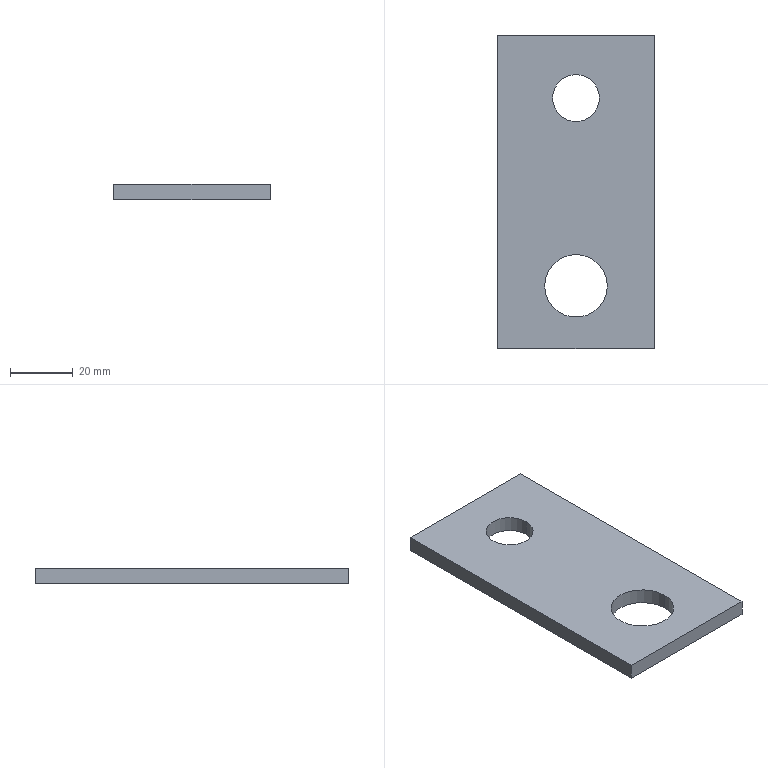Part | SolidWorks | features Extrusion 1, ICE 1 | 1 solid | 10 faces | box 50 x 100 x 5 mm | volume 22546 mm3 | plane 6 | cylinder 4 | commonest cylinder face diameters 15 x2 20 x2
STEP:
#1=CARTESIAN_POINT('',(-7.5,30.,0.));
#2=VERTEX_POINT('',#1);
#3=CARTESIAN_POINT('',(7.5,30.,0.));
#4=VERTEX_POINT('',#3);
#5=CARTESIAN_POINT('',(0.,30.,0.));
#6=DIRECTION('',(0.,0.,1.));
#7=DIRECTION('',(1.,0.,0.));
#8=AXIS2_PLACEMENT_3D('',#5,#6,#7);
#9=CIRCLE('',#8,7.5);
#10=EDGE_CURVE('',#2,#4,#9,.T.);
#11=ORIENTED_EDGE('',*,*,#10,.F.);
#12=CARTESIAN_POINT('',(-7.5,30.,5.));
#13=VERTEX_POINT('',#12);
#14=CARTESIAN_POINT('',(-7.5,30.,0.));
#15=DIRECTION('',(0.,0.,1.));
#16=VECTOR('',#15,1000.);
#17=LINE('',#14,#16);
#18=EDGE_CURVE('',#2,#13,#17,.T.);
#19=ORIENTED_EDGE('',*,*,#18,.T.);
#20=CARTESIAN_POINT('',(7.5,30.,5.));
#21=VERTEX_POINT('',#20);
#22=CARTESIAN_POINT('',(0.,30.,5.));
#23=DIRECTION('',(0.,0.,1.));
#24=DIRECTION('',(1.,0.,0.));
#25=AXIS2_PLACEMENT_3D('',#22,#23,#24);
#26=CIRCLE('',#25,7.5);
#27=EDGE_CURVE('',#13,#21,#26,.T.);
#28=ORIENTED_EDGE('',*,*,#27,.T.);
#29=CARTESIAN_POINT('',(7.5,30.,0.));
#30=DIRECTION('',(0.,0.,1.));
#31=VECTOR('',#30,1000.);
#32=LINE('',#29,#31);
#33=EDGE_CURVE('',#4,#21,#32,.T.);
#34=ORIENTED_EDGE('',*,*,#33,.F.);
#35=EDGE_LOOP('',(#11,#19,#28,#34));
#36=FACE_OUTER_BOUND('',#35,.T.);
#37=CARTESIAN_POINT('',(0.,30.,0.));
#38=DIRECTION('',(0.,0.,1.));
#39=DIRECTION('',(1.,0.,0.));
#40=AXIS2_PLACEMENT_3D('',#37,#38,#39);
#41=CYLINDRICAL_SURFACE('',#40,7.5);
#42=ADVANCED_FACE('',(#36),#41,.F.);
#43=CARTESIAN_POINT('',(-10.,-30.,0.));
#44=VERTEX_POINT('',#43);
#45=CARTESIAN_POINT('',(10.,-30.,0.));
#46=VERTEX_POINT('',#45);
#47=CARTESIAN_POINT('',(0.,-30.,0.));
#48=DIRECTION('',(0.,0.,1.));
#49=DIRECTION('',(1.,0.,0.));
#50=AXIS2_PLACEMENT_3D('',#47,#48,#49);
#51=CIRCLE('',#50,10.);
#52=EDGE_CURVE('',#44,#46,#51,.T.);
#53=ORIENTED_EDGE('',*,*,#52,.F.);
#54=CARTESIAN_POINT('',(-10.,-30.,5.));
#55=VERTEX_POINT('',#54);
#56=CARTESIAN_POINT('',(-10.,-30.,0.));
#57=DIRECTION('',(0.,0.,1.));
#58=VECTOR('',#57,1000.);
#59=LINE('',#56,#58);
#60=EDGE_CURVE('',#44,#55,#59,.T.);
#61=ORIENTED_EDGE('',*,*,#60,.T.);
#62=CARTESIAN_POINT('',(10.,-30.,5.));
#63=VERTEX_POINT('',#62);
#64=CARTESIAN_POINT('',(0.,-30.,5.));
#65=DIRECTION('',(0.,0.,1.));
#66=DIRECTION('',(1.,0.,0.));
#67=AXIS2_PLACEMENT_3D('',#64,#65,#66);
#68=CIRCLE('',#67,10.);
#69=EDGE_CURVE('',#55,#63,#68,.T.);
#70=ORIENTED_EDGE('',*,*,#69,.T.);
#71=CARTESIAN_POINT('',(10.,-30.,0.));
#72=DIRECTION('',(0.,0.,1.));
#73=VECTOR('',#72,1000.);
#74=LINE('',#71,#73);
#75=EDGE_CURVE('',#46,#63,#74,.T.);
#76=ORIENTED_EDGE('',*,*,#75,.F.);
#77=EDGE_LOOP('',(#53,#61,#70,#76));
#78=FACE_OUTER_BOUND('',#77,.T.);
#79=CARTESIAN_POINT('',(0.,-30.,0.));
#80=DIRECTION('',(0.,0.,1.));
#81=DIRECTION('',(1.,0.,0.));
#82=AXIS2_PLACEMENT_3D('',#79,#80,#81);
#83=CYLINDRICAL_SURFACE('',#82,10.);
#84=ADVANCED_FACE('',(#78),#83,.F.);
#85=CARTESIAN_POINT('',(-25.,50.,0.));
#86=VERTEX_POINT('',#85);
#87=CARTESIAN_POINT('',(-25.,-50.,0.));
#88=VERTEX_POINT('',#87);
#89=CARTESIAN_POINT('',(-25.,50.,0.));
#90=DIRECTION('',(0.,-1.,0.));
#91=VECTOR('',#90,1000.);
#92=LINE('',#89,#91);
#93=EDGE_CURVE('',#86,#88,#92,.T.);
#94=ORIENTED_EDGE('',*,*,#93,.T.);
#95=CARTESIAN_POINT('',(-25.,-50.,5.));
#96=VERTEX_POINT('',#95);
#97=CARTESIAN_POINT('',(-25.,-50.,5.));
#98=DIRECTION('',(0.,0.,-1.));
#99=VECTOR('',#98,1000.);
#100=LINE('',#97,#99);
#101=EDGE_CURVE('',#96,#88,#100,.T.);
#102=ORIENTED_EDGE('',*,*,#101,.F.);
#103=CARTESIAN_POINT('',(-25.,50.,5.));
#104=VERTEX_POINT('',#103);
#105=CARTESIAN_POINT('',(-25.,50.,5.));
#106=DIRECTION('',(0.,-1.,0.));
#107=VECTOR('',#106,1000.);
#108=LINE('',#105,#107);
#109=EDGE_CURVE('',#104,#96,#108,.T.);
#110=ORIENTED_EDGE('',*,*,#109,.F.);
#111=CARTESIAN_POINT('',(-25.,50.,5.));
#112=DIRECTION('',(0.,0.,-1.));
#113=VECTOR('',#112,1000.);
#114=LINE('',#111,#113);
#115=EDGE_CURVE('',#104,#86,#114,.T.);
#116=ORIENTED_EDGE('',*,*,#115,.T.);
#117=EDGE_LOOP('',(#94,#102,#110,#116));
#118=FACE_OUTER_BOUND('',#117,.T.);
#119=CARTESIAN_POINT('',(-25.,50.,5.));
#120=DIRECTION('',(1.,0.,0.));
#121=DIRECTION('',(0.,1.,0.));
#122=AXIS2_PLACEMENT_3D('',#119,#120,#121);
#123=PLANE('',#122);
#124=ADVANCED_FACE('',(#118),#123,.F.);
#125=CARTESIAN_POINT('',(25.,-50.,0.));
#126=VERTEX_POINT('',#125);
#127=CARTESIAN_POINT('',(25.,-50.,0.));
#128=DIRECTION('',(1.,0.,0.));
#129=VECTOR('',#128,1000.);
#130=LINE('',#127,#129);
#131=EDGE_CURVE('',#88,#126,#130,.T.);
#132=ORIENTED_EDGE('',*,*,#131,.T.);
#133=CARTESIAN_POINT('',(25.,-50.,5.));
#134=VERTEX_POINT('',#133);
#135=CARTESIAN_POINT('',(25.,-50.,5.));
#136=DIRECTION('',(0.,0.,-1.));
#137=VECTOR('',#136,1000.);
#138=LINE('',#135,#137);
#139=EDGE_CURVE('',#134,#126,#138,.T.);
#140=ORIENTED_EDGE('',*,*,#139,.F.);
#141=CARTESIAN_POINT('',(25.,-50.,5.));
#142=DIRECTION('',(1.,0.,0.));
#143=VECTOR('',#142,1000.);
#144=LINE('',#141,#143);
#145=EDGE_CURVE('',#96,#134,#144,.T.);
#146=ORIENTED_EDGE('',*,*,#145,.F.);
#147=ORIENTED_EDGE('',*,*,#101,.T.);
#148=EDGE_LOOP('',(#132,#140,#146,#147));
#149=FACE_OUTER_BOUND('',#148,.T.);
#150=CARTESIAN_POINT('',(25.,-50.,5.));
#151=DIRECTION('',(0.,1.,0.));
#152=DIRECTION('',(0.,0.,1.));
#153=AXIS2_PLACEMENT_3D('',#150,#151,#152);
#154=PLANE('',#153);
#155=ADVANCED_FACE('',(#149),#154,.F.);
#156=CARTESIAN_POINT('',(25.,50.,0.));
#157=VERTEX_POINT('',#156);
#158=CARTESIAN_POINT('',(25.,50.,0.));
#159=DIRECTION('',(0.,1.,0.));
#160=VECTOR('',#159,1000.);
#161=LINE('',#158,#160);
#162=EDGE_CURVE('',#126,#157,#161,.T.);
#163=ORIENTED_EDGE('',*,*,#162,.T.);
#164=CARTESIAN_POINT('',(25.,50.,5.));
#165=VERTEX_POINT('',#164);
#166=CARTESIAN_POINT('',(25.,50.,5.));
#167=DIRECTION('',(0.,0.,-1.));
#168=VECTOR('',#167,1000.);
#169=LINE('',#166,#168);
#170=EDGE_CURVE('',#165,#157,#169,.T.);
#171=ORIENTED_EDGE('',*,*,#170,.F.);
#172=CARTESIAN_POINT('',(25.,50.,5.));
#173=DIRECTION('',(0.,1.,0.));
#174=VECTOR('',#173,1000.);
#175=LINE('',#172,#174);
#176=EDGE_CURVE('',#134,#165,#175,.T.);
#177=ORIENTED_EDGE('',*,*,#176,.F.);
#178=ORIENTED_EDGE('',*,*,#139,.T.);
#179=EDGE_LOOP('',(#163,#171,#177,#178));
#180=FACE_OUTER_BOUND('',#179,.T.);
#181=CARTESIAN_POINT('',(25.,50.,5.));
#182=DIRECTION('',(-1.,0.,0.));
#183=DIRECTION('',(0.,-1.,0.));
#184=AXIS2_PLACEMENT_3D('',#181,#182,#183);
#185=PLANE('',#184);
#186=ADVANCED_FACE('',(#180),#185,.F.);
#187=CARTESIAN_POINT('',(25.,50.,0.));
#188=DIRECTION('',(-1.,0.,0.));
#189=VECTOR('',#188,1000.);
#190=LINE('',#187,#189);
#191=EDGE_CURVE('',#157,#86,#190,.T.);
#192=ORIENTED_EDGE('',*,*,#191,.T.);
#193=ORIENTED_EDGE('',*,*,#115,.F.);
#194=CARTESIAN_POINT('',(25.,50.,5.));
#195=DIRECTION('',(-1.,0.,0.));
#196=VECTOR('',#195,1000.);
#197=LINE('',#194,#196);
#198=EDGE_CURVE('',#165,#104,#197,.T.);
#199=ORIENTED_EDGE('',*,*,#198,.F.);
#200=ORIENTED_EDGE('',*,*,#170,.T.);
#201=EDGE_LOOP('',(#192,#193,#199,#200));
#202=FACE_OUTER_BOUND('',#201,.T.);
#203=CARTESIAN_POINT('',(25.,50.,5.));
#204=DIRECTION('',(0.,-1.,0.));
#205=DIRECTION('',(0.,0.,-1.));
#206=AXIS2_PLACEMENT_3D('',#203,#204,#205);
#207=PLANE('',#206);
#208=ADVANCED_FACE('',(#202),#207,.F.);
#209=CARTESIAN_POINT('',(0.,30.,5.));
#210=DIRECTION('',(0.,0.,1.));
#211=DIRECTION('',(1.,0.,0.));
#212=AXIS2_PLACEMENT_3D('',#209,#210,#211);
#213=CIRCLE('',#212,7.5);
#214=EDGE_CURVE('',#21,#13,#213,.T.);
#215=ORIENTED_EDGE('',*,*,#214,.F.);
#216=ORIENTED_EDGE('',*,*,#27,.F.);
#217=EDGE_LOOP('',(#215,#216));
#218=FACE_BOUND('',#217,.T.);
#219=CARTESIAN_POINT('',(0.,-30.,5.));
#220=DIRECTION('',(0.,0.,1.));
#221=DIRECTION('',(1.,0.,0.));
#222=AXIS2_PLACEMENT_3D('',#219,#220,#221);
#223=CIRCLE('',#222,10.);
#224=EDGE_CURVE('',#63,#55,#223,.T.);
#225=ORIENTED_EDGE('',*,*,#224,.F.);
#226=ORIENTED_EDGE('',*,*,#69,.F.);
#227=EDGE_LOOP('',(#225,#226));
#228=FACE_BOUND('',#227,.T.);
#229=ORIENTED_EDGE('',*,*,#109,.T.);
#230=ORIENTED_EDGE('',*,*,#145,.T.);
#231=ORIENTED_EDGE('',*,*,#176,.T.);
#232=ORIENTED_EDGE('',*,*,#198,.T.);
#233=EDGE_LOOP('',(#229,#230,#231,#232));
#234=FACE_OUTER_BOUND('',#233,.T.);
#235=CARTESIAN_POINT('',(0.,0.,5.));
#236=DIRECTION('',(0.,0.,-1.));
#237=DIRECTION('',(-1.,0.,0.));
#238=AXIS2_PLACEMENT_3D('',#235,#236,#237);
#239=PLANE('',#238);
#240=ADVANCED_FACE('',(#218,#228,#234),#239,.F.);
#241=CARTESIAN_POINT('',(0.,30.,0.));
#242=DIRECTION('',(0.,0.,1.));
#243=DIRECTION('',(1.,0.,0.));
#244=AXIS2_PLACEMENT_3D('',#241,#242,#243);
#245=CIRCLE('',#244,7.5);
#246=EDGE_CURVE('',#4,#2,#245,.T.);
#247=ORIENTED_EDGE('',*,*,#246,.T.);
#248=ORIENTED_EDGE('',*,*,#10,.T.);
#249=EDGE_LOOP('',(#247,#248));
#250=FACE_BOUND('',#249,.T.);
#251=CARTESIAN_POINT('',(0.,-30.,0.));
#252=DIRECTION('',(0.,0.,1.));
#253=DIRECTION('',(1.,0.,0.));
#254=AXIS2_PLACEMENT_3D('',#251,#252,#253);
#255=CIRCLE('',#254,10.);
#256=EDGE_CURVE('',#46,#44,#255,.T.);
#257=ORIENTED_EDGE('',*,*,#256,.T.);
#258=ORIENTED_EDGE('',*,*,#52,.T.);
#259=EDGE_LOOP('',(#257,#258));
#260=FACE_BOUND('',#259,.T.);
#261=ORIENTED_EDGE('',*,*,#93,.F.);
#262=ORIENTED_EDGE('',*,*,#191,.F.);
#263=ORIENTED_EDGE('',*,*,#162,.F.);
#264=ORIENTED_EDGE('',*,*,#131,.F.);
#265=EDGE_LOOP('',(#261,#262,#263,#264));
#266=FACE_OUTER_BOUND('',#265,.T.);
#267=CARTESIAN_POINT('',(0.,0.,0.));
#268=DIRECTION('',(0.,0.,-1.));
#269=DIRECTION('',(-1.,0.,0.));
#270=AXIS2_PLACEMENT_3D('',#267,#268,#269);
#271=PLANE('',#270);
#272=ADVANCED_FACE('',(#250,#260,#266),#271,.T.);
#273=ORIENTED_EDGE('',*,*,#60,.F.);
#274=ORIENTED_EDGE('',*,*,#256,.F.);
#275=ORIENTED_EDGE('',*,*,#75,.T.);
#276=ORIENTED_EDGE('',*,*,#224,.T.);
#277=EDGE_LOOP('',(#273,#274,#275,#276));
#278=FACE_OUTER_BOUND('',#277,.T.);
#279=CARTESIAN_POINT('',(0.,-30.,0.));
#280=DIRECTION('',(0.,0.,1.));
#281=DIRECTION('',(1.,0.,0.));
#282=AXIS2_PLACEMENT_3D('',#279,#280,#281);
#283=CYLINDRICAL_SURFACE('',#282,10.);
#284=ADVANCED_FACE('',(#278),#283,.F.);
#285=ORIENTED_EDGE('',*,*,#18,.F.);
#286=ORIENTED_EDGE('',*,*,#246,.F.);
#287=ORIENTED_EDGE('',*,*,#33,.T.);
#288=ORIENTED_EDGE('',*,*,#214,.T.);
#289=EDGE_LOOP('',(#285,#286,#287,#288));
#290=FACE_OUTER_BOUND('',#289,.T.);
#291=CARTESIAN_POINT('',(0.,30.,0.));
#292=DIRECTION('',(0.,0.,1.));
#293=DIRECTION('',(1.,0.,0.));
#294=AXIS2_PLACEMENT_3D('',#291,#292,#293);
#295=CYLINDRICAL_SURFACE('',#294,7.5);
#296=ADVANCED_FACE('',(#290),#295,.F.);
#297=CLOSED_SHELL('',(#42,#84,#124,#155,#186,#208,#240,#272,#284,#296));
#298=MANIFOLD_SOLID_BREP('',#297);
#299=CARTESIAN_POINT('',(0.,0.,0.));
#300=DIRECTION('',(0.,0.,1.));
#301=DIRECTION('',(1.,0.,0.));
#302=AXIS2_PLACEMENT_3D('',#299,#300,#301);
#303=(LENGTH_UNIT()NAMED_UNIT(*)SI_UNIT(.MILLI.,.METRE.));
#304=UNCERTAINTY_MEASURE_WITH_UNIT(LENGTH_MEASURE(0.00001),#303,'','');
#305=(NAMED_UNIT(*)PLANE_ANGLE_UNIT()SI_UNIT($,.RADIAN.));
#306=(NAMED_UNIT(*)SI_UNIT($,.STERADIAN.)SOLID_ANGLE_UNIT());
#307=(GEOMETRIC_REPRESENTATION_CONTEXT(3)GLOBAL_UNCERTAINTY_ASSIGNED_CONTEXT((#304))GLOBAL_UNIT_ASSIGNED_CONTEXT((#303,#305,#306))REPRESENTATION_CONTEXT('',''));
#308=ADVANCED_BREP_SHAPE_REPRESENTATION('',(#298,#302),#307);